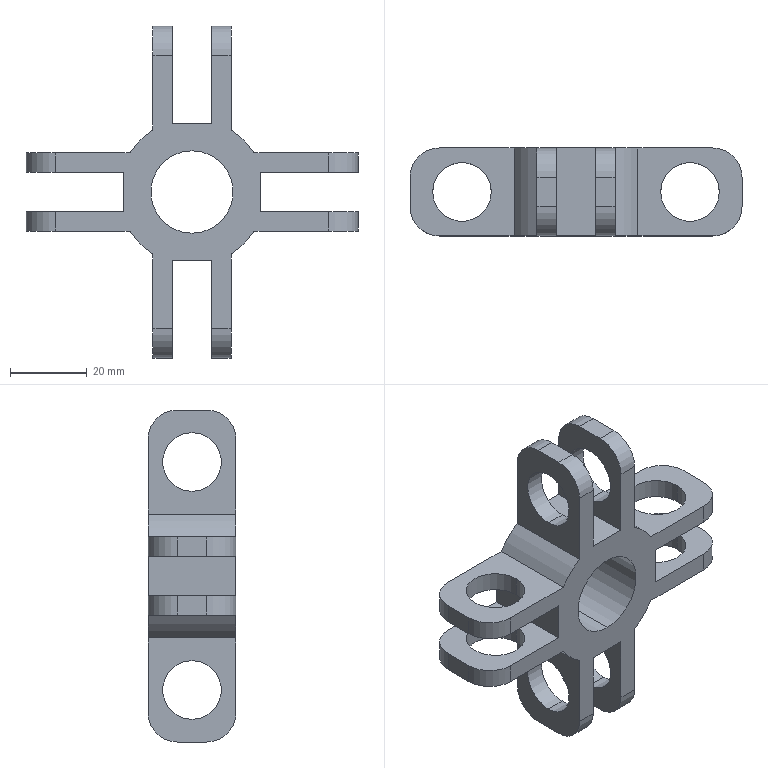Part | SolidWorks | features ICE 4, CirPattern 1, Extrusion 1, Fillet 1, HoleWzd 1, Scale 1 | 1 solid | 68 faces | box 86.36 x 22.86 x 86.36 mm | volume 32385 mm3 | cylinder 38 | plane 30 | commonest cylinder face diameters 15.24 x32 38.1 x4 21.433 x2